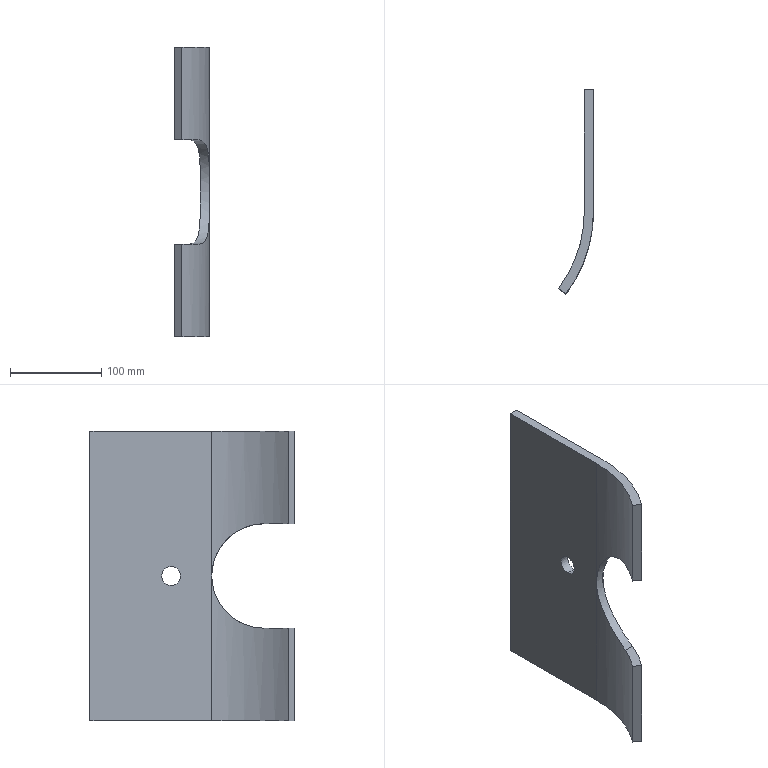Part | SolidWorks | features Extrusion 1, ICE 1 | 1 solid | 16 faces | box 38.131 x 223.442 x 317.5 mm | volume 624053 mm3 | plane 9 | cylinder 7 | commonest cylinder face diameters 20.574 x2 279.4 x2 299.4 x2 114.3 x1
STEP:
#1=CARTESIAN_POINT('',(-10.,0.,10.287));
#2=VERTEX_POINT('',#1);
#3=CARTESIAN_POINT('',(-10.,0.,-10.287));
#4=VERTEX_POINT('',#3);
#5=CARTESIAN_POINT('',(-10.,0.,0.));
#6=DIRECTION('',(1.,0.,0.));
#7=DIRECTION('',(0.,1.,0.));
#8=AXIS2_PLACEMENT_3D('',#5,#6,#7);
#9=CIRCLE('',#8,10.287);
#10=EDGE_CURVE('',#2,#4,#9,.T.);
#11=ORIENTED_EDGE('',*,*,#10,.F.);
#12=CARTESIAN_POINT('',(0.,0.,10.287));
#13=VERTEX_POINT('',#12);
#14=CARTESIAN_POINT('',(-184.15,0.,10.287));
#15=DIRECTION('',(1.,0.,0.));
#16=VECTOR('',#15,1000.);
#17=LINE('',#14,#16);
#18=EDGE_CURVE('',#2,#13,#17,.T.);
#19=ORIENTED_EDGE('',*,*,#18,.T.);
#20=CARTESIAN_POINT('',(0.,0.,-10.287));
#21=VERTEX_POINT('',#20);
#22=CARTESIAN_POINT('',(0.,0.,0.));
#23=DIRECTION('',(-1.,0.,0.));
#24=DIRECTION('',(0.,-1.,0.));
#25=AXIS2_PLACEMENT_3D('',#22,#23,#24);
#26=CIRCLE('',#25,10.287);
#27=EDGE_CURVE('',#21,#13,#26,.T.);
#28=ORIENTED_EDGE('',*,*,#27,.F.);
#29=CARTESIAN_POINT('',(-184.15,0.,-10.287));
#30=DIRECTION('',(1.,0.,0.));
#31=VECTOR('',#30,1000.);
#32=LINE('',#29,#31);
#33=EDGE_CURVE('',#4,#21,#32,.T.);
#34=ORIENTED_EDGE('',*,*,#33,.F.);
#35=EDGE_LOOP('',(#11,#19,#28,#34));
#36=FACE_OUTER_BOUND('',#35,.T.);
#37=CARTESIAN_POINT('',(-184.15,0.,0.));
#38=DIRECTION('',(1.,0.,0.));
#39=DIRECTION('',(0.,0.,-1.));
#40=AXIS2_PLACEMENT_3D('',#37,#38,#39);
#41=CYLINDRICAL_SURFACE('',#40,10.287);
#42=ADVANCED_FACE('',(#36),#41,.F.);
#43=CARTESIAN_POINT('',(-38.131,-128.524,-57.15));
#44=VERTEX_POINT('',#43);
#45=CARTESIAN_POINT('',(-38.131,-128.524,-158.75));
#46=VERTEX_POINT('',#45);
#47=CARTESIAN_POINT('',(-38.131,-128.524,158.75));
#48=DIRECTION('',(0.,0.,-1.));
#49=VECTOR('',#48,1000.);
#50=LINE('',#47,#49);
#51=EDGE_CURVE('',#44,#46,#50,.T.);
#52=ORIENTED_EDGE('',*,*,#51,.F.);
#53=CARTESIAN_POINT('',(-22.225,-101.6,-57.15));
#54=VERTEX_POINT('',#53);
#55=CARTESIAN_POINT('',(-149.7,-44.45,-57.15));
#56=DIRECTION('',(0.,0.,1.));
#57=DIRECTION('',(0.,1.,0.));
#58=AXIS2_PLACEMENT_3D('',#55,#56,#57);
#59=CIRCLE('',#58,139.7);
#60=EDGE_CURVE('',#44,#54,#59,.T.);
#61=ORIENTED_EDGE('',*,*,#60,.T.);
#62=CARTESIAN_POINT('',(-10.,-44.45,0.));
#63=VERTEX_POINT('',#62);
#64=CARTESIAN_POINT('',(-22.225,-101.6,-57.15));
#65=CARTESIAN_POINT('',(-20.653,-98.094,-57.15));
#66=CARTESIAN_POINT('',(-19.249,-94.576,-56.83));
#67=CARTESIAN_POINT('',(-17.38,-89.293,-55.838));
#68=CARTESIAN_POINT('',(-16.796,-87.531,-55.422));
#69=CARTESIAN_POINT('',(-15.978,-84.889,-54.66));
#70=CARTESIAN_POINT('',(-15.714,-84.006,-54.382));
#71=CARTESIAN_POINT('',(-15.209,-82.255,-53.784));
#72=CARTESIAN_POINT('',(-14.969,-81.387,-53.464));
#73=CARTESIAN_POINT('',(-13.82,-77.092,-51.76));
#74=CARTESIAN_POINT('',(-13.077,-73.786,-50.067));
#75=CARTESIAN_POINT('',(-12.324,-69.838,-47.52));
#76=CARTESIAN_POINT('',(-12.182,-69.057,-46.989));
#77=CARTESIAN_POINT('',(-11.915,-67.516,-45.883));
#78=CARTESIAN_POINT('',(-11.79,-66.753,-45.307));
#79=CARTESIAN_POINT('',(-11.441,-64.523,-43.532));
#80=CARTESIAN_POINT('',(-11.244,-63.102,-42.28));
#81=CARTESIAN_POINT('',(-10.906,-60.393,-39.644));
#82=CARTESIAN_POINT('',(-10.765,-59.104,-38.259));
#83=CARTESIAN_POINT('',(-10.588,-57.27,-36.082));
#84=CARTESIAN_POINT('',(-10.535,-56.676,-35.339));
#85=CARTESIAN_POINT('',(-10.438,-55.522,-33.82));
#86=CARTESIAN_POINT('',(-10.395,-54.96,-33.042));
#87=CARTESIAN_POINT('',(-10.201,-52.253,-29.081));
#88=CARTESIAN_POINT('',(-10.12,-50.436,-25.745));
#89=CARTESIAN_POINT('',(-10.049,-48.219,-20.499));
#90=CARTESIAN_POINT('',(-10.034,-47.565,-18.709));
#91=CARTESIAN_POINT('',(-10.018,-46.716,-15.963));
#92=CARTESIAN_POINT('',(-10.014,-46.455,-15.036));
#93=CARTESIAN_POINT('',(-10.008,-45.983,-13.181));
#94=CARTESIAN_POINT('',(-10.006,-45.77,-12.251));
#95=CARTESIAN_POINT('',(-9.998,-44.828,-7.588));
#96=CARTESIAN_POINT('',(-10.,-44.45,-3.815));
#97=CARTESIAN_POINT('',(-10.,-44.45,0.));
#98=B_SPLINE_CURVE_WITH_KNOTS('',3,(#64,#65,#66,#67,#68,#69,#70,#71,#72,#73,#74,#75,#76,#77,#78,#79,#80,#81,#82,#83,#84,#85,#86,#87,#88,#89,#90,#91,#92,#93,#94,#95,#96,#97),.UNSPECIFIED.,.F.,.F.,(4,2,2,2,2,2,2,2,2,2,2,2,2,2,2,2,4),(0.,0.01138,0.01706,0.01991,0.02275,0.03413,0.03697,0.03982,0.0455,0.05119,0.05404,0.05688,0.06826,0.07394,0.07679,0.07963,0.09101),.UNSPECIFIED.);
#99=EDGE_CURVE('',#54,#63,#98,.T.);
#100=ORIENTED_EDGE('',*,*,#99,.T.);
#101=CARTESIAN_POINT('',(-10.,-44.45,-158.75));
#102=VERTEX_POINT('',#101);
#103=CARTESIAN_POINT('',(-10.,-44.45,158.75));
#104=DIRECTION('',(0.,0.,-1.));
#105=VECTOR('',#104,1000.);
#106=LINE('',#103,#105);
#107=EDGE_CURVE('',#63,#102,#106,.T.);
#108=ORIENTED_EDGE('',*,*,#107,.T.);
#109=CARTESIAN_POINT('',(-149.7,-44.45,-158.75));
#110=DIRECTION('',(0.,0.,-1.));
#111=DIRECTION('',(1.,0.,0.));
#112=AXIS2_PLACEMENT_3D('',#109,#110,#111);
#113=CIRCLE('',#112,139.7);
#114=EDGE_CURVE('',#102,#46,#113,.T.);
#115=ORIENTED_EDGE('',*,*,#114,.T.);
#116=EDGE_LOOP('',(#52,#61,#100,#108,#115));
#117=FACE_OUTER_BOUND('',#116,.T.);
#118=CARTESIAN_POINT('',(-149.7,-44.45,158.75));
#119=DIRECTION('',(0.,0.,-1.));
#120=DIRECTION('',(-1.,0.,0.));
#121=AXIS2_PLACEMENT_3D('',#118,#119,#120);
#122=CYLINDRICAL_SURFACE('',#121,139.7);
#123=ADVANCED_FACE('',(#117),#122,.F.);
#124=CARTESIAN_POINT('',(-30.144,-134.542,-57.15));
#125=VERTEX_POINT('',#124);
#126=CARTESIAN_POINT('',(-30.144,-134.542,-158.75));
#127=VERTEX_POINT('',#126);
#128=CARTESIAN_POINT('',(-30.144,-134.542,158.75));
#129=DIRECTION('',(0.,0.,-1.));
#130=VECTOR('',#129,1000.);
#131=LINE('',#128,#130);
#132=EDGE_CURVE('',#125,#127,#131,.T.);
#133=ORIENTED_EDGE('',*,*,#132,.F.);
#134=CARTESIAN_POINT('',(-30.144,-134.542,-57.15));
#135=DIRECTION('',(-0.7986,0.6018,0.));
#136=VECTOR('',#135,1000.);
#137=LINE('',#134,#136);
#138=EDGE_CURVE('',#125,#44,#137,.T.);
#139=ORIENTED_EDGE('',*,*,#138,.T.);
#140=ORIENTED_EDGE('',*,*,#51,.T.);
#141=CARTESIAN_POINT('',(-30.144,-134.542,-158.75));
#142=DIRECTION('',(0.7986,-0.6018,0.));
#143=VECTOR('',#142,1000.);
#144=LINE('',#141,#143);
#145=EDGE_CURVE('',#46,#127,#144,.T.);
#146=ORIENTED_EDGE('',*,*,#145,.T.);
#147=EDGE_LOOP('',(#133,#139,#140,#146));
#148=FACE_OUTER_BOUND('',#147,.T.);
#149=CARTESIAN_POINT('',(-30.144,-134.542,158.75));
#150=DIRECTION('',(0.6018,0.7986,0.));
#151=DIRECTION('',(-0.7986,0.6018,0.));
#152=AXIS2_PLACEMENT_3D('',#149,#150,#151);
#153=PLANE('',#152);
#154=ADVANCED_FACE('',(#148),#153,.F.);
#155=CARTESIAN_POINT('',(0.,-44.45,0.));
#156=VERTEX_POINT('',#155);
#157=CARTESIAN_POINT('',(-11.338,-101.6,-57.15));
#158=VERTEX_POINT('',#157);
#159=CARTESIAN_POINT('',(0.,-44.45,0.));
#160=CARTESIAN_POINT('',(0.,-44.45,-0.9496));
#161=CARTESIAN_POINT('',(0.000005753,-44.474,-1.902));
#162=CARTESIAN_POINT('',(-0.00003983,-44.569,-3.811));
#163=CARTESIAN_POINT('',(-0.00009177,-44.641,-4.767));
#164=CARTESIAN_POINT('',(-0.0006387,-44.927,-7.611));
#165=CARTESIAN_POINT('',(-0.001464,-45.211,-9.485));
#166=CARTESIAN_POINT('',(-0.009996,-46.335,-15.041));
#167=CARTESIAN_POINT('',(-0.0226,-47.446,-18.66));
#168=CARTESIAN_POINT('',(-0.08943,-49.677,-23.954));
#169=CARTESIAN_POINT('',(-0.1197,-50.504,-25.669));
#170=CARTESIAN_POINT('',(-0.204,-52.314,-28.994));
#171=CARTESIAN_POINT('',(-0.2579,-53.298,-30.605));
#172=CARTESIAN_POINT('',(-0.3989,-55.423,-33.725));
#173=CARTESIAN_POINT('',(-0.4859,-56.564,-35.235));
#174=CARTESIAN_POINT('',(-0.6497,-58.395,-37.421));
#175=CARTESIAN_POINT('',(-0.7099,-59.027,-38.139));
#176=CARTESIAN_POINT('',(-0.8426,-60.324,-39.539));
#177=CARTESIAN_POINT('',(-0.9146,-60.987,-40.219));
#178=CARTESIAN_POINT('',(-1.307,-64.373,-43.527));
#179=CARTESIAN_POINT('',(-1.72,-67.305,-45.87));
#180=CARTESIAN_POINT('',(-2.414,-71.237,-48.426));
#181=CARTESIAN_POINT('',(-2.562,-72.037,-48.919));
#182=CARTESIAN_POINT('',(-2.876,-73.664,-49.866));
#183=CARTESIAN_POINT('',(-3.043,-74.493,-50.321));
#184=CARTESIAN_POINT('',(-3.57,-76.993,-51.615));
#185=CARTESIAN_POINT('',(-3.956,-78.683,-52.386));
#186=CARTESIAN_POINT('',(-5.226,-83.817,-54.438));
#187=CARTESIAN_POINT('',(-6.222,-87.325,-55.459));
#188=CARTESIAN_POINT('',(-7.976,-92.7,-56.482));
#189=CARTESIAN_POINT('',(-8.598,-94.489,-56.734));
#190=CARTESIAN_POINT('',(-9.913,-98.053,-57.068));
#191=CARTESIAN_POINT('',(-10.607,-99.83,-57.15));
#192=CARTESIAN_POINT('',(-11.338,-101.6,-57.15));
#193=B_SPLINE_CURVE_WITH_KNOTS('',3,(#159,#160,#161,#162,#163,#164,#165,#166,#167,#168,#169,#170,#171,#172,#173,#174,#175,#176,#177,#178,#179,#180,#181,#182,#183,#184,#185,#186,#187,#188,#189,#190,#191,#192),.UNSPECIFIED.,.F.,.F.,(4,2,2,2,2,2,2,2,2,2,2,2,2,2,2,2,4),(0.09078,0.09361,0.09645,0.1021,0.1135,0.1191,0.1248,0.1305,0.1333,0.1361,0.1475,0.1503,0.1531,0.1588,0.1701,0.1758,0.1815),.UNSPECIFIED.);
#194=EDGE_CURVE('',#156,#158,#193,.T.);
#195=ORIENTED_EDGE('',*,*,#194,.T.);
#196=CARTESIAN_POINT('',(-149.7,-44.45,-57.15));
#197=DIRECTION('',(0.,0.,-1.));
#198=DIRECTION('',(0.,1.,0.));
#199=AXIS2_PLACEMENT_3D('',#196,#197,#198);
#200=CIRCLE('',#199,149.7);
#201=EDGE_CURVE('',#158,#125,#200,.T.);
#202=ORIENTED_EDGE('',*,*,#201,.T.);
#203=ORIENTED_EDGE('',*,*,#132,.T.);
#204=CARTESIAN_POINT('',(0.,-44.45,-158.75));
#205=VERTEX_POINT('',#204);
#206=CARTESIAN_POINT('',(-149.7,-44.45,-158.75));
#207=DIRECTION('',(0.,0.,1.));
#208=DIRECTION('',(1.,0.,0.));
#209=AXIS2_PLACEMENT_3D('',#206,#207,#208);
#210=CIRCLE('',#209,149.7);
#211=EDGE_CURVE('',#127,#205,#210,.T.);
#212=ORIENTED_EDGE('',*,*,#211,.T.);
#213=CARTESIAN_POINT('',(0.,-44.45,158.75));
#214=DIRECTION('',(0.,0.,-1.));
#215=VECTOR('',#214,1000.);
#216=LINE('',#213,#215);
#217=EDGE_CURVE('',#156,#205,#216,.T.);
#218=ORIENTED_EDGE('',*,*,#217,.F.);
#219=EDGE_LOOP('',(#195,#202,#203,#212,#218));
#220=FACE_OUTER_BOUND('',#219,.T.);
#221=CARTESIAN_POINT('',(-149.7,-44.45,158.75));
#222=DIRECTION('',(0.,0.,-1.));
#223=DIRECTION('',(-1.,0.,0.));
#224=AXIS2_PLACEMENT_3D('',#221,#222,#223);
#225=CYLINDRICAL_SURFACE('',#224,149.7);
#226=ADVANCED_FACE('',(#220),#225,.T.);
#227=CARTESIAN_POINT('',(-10.,0.,0.));
#228=DIRECTION('',(1.,0.,0.));
#229=DIRECTION('',(0.,1.,0.));
#230=AXIS2_PLACEMENT_3D('',#227,#228,#229);
#231=CIRCLE('',#230,10.287);
#232=EDGE_CURVE('',#4,#2,#231,.T.);
#233=ORIENTED_EDGE('',*,*,#232,.T.);
#234=ORIENTED_EDGE('',*,*,#10,.T.);
#235=EDGE_LOOP('',(#233,#234));
#236=FACE_BOUND('',#235,.T.);
#237=CARTESIAN_POINT('',(-10.,88.9,-158.75));
#238=VERTEX_POINT('',#237);
#239=CARTESIAN_POINT('',(-10.,88.9,-158.75));
#240=DIRECTION('',(0.,-1.,0.));
#241=VECTOR('',#240,1000.);
#242=LINE('',#239,#241);
#243=EDGE_CURVE('',#238,#102,#242,.T.);
#244=ORIENTED_EDGE('',*,*,#243,.T.);
#245=ORIENTED_EDGE('',*,*,#107,.F.);
#246=CARTESIAN_POINT('',(-10.,-44.45,158.75));
#247=VERTEX_POINT('',#246);
#248=CARTESIAN_POINT('',(-10.,-44.45,158.75));
#249=DIRECTION('',(0.,0.,-1.));
#250=VECTOR('',#249,1000.);
#251=LINE('',#248,#250);
#252=EDGE_CURVE('',#247,#63,#251,.T.);
#253=ORIENTED_EDGE('',*,*,#252,.F.);
#254=CARTESIAN_POINT('',(-10.,88.9,158.75));
#255=VERTEX_POINT('',#254);
#256=CARTESIAN_POINT('',(-10.,88.9,158.75));
#257=DIRECTION('',(0.,-1.,0.));
#258=VECTOR('',#257,1000.);
#259=LINE('',#256,#258);
#260=EDGE_CURVE('',#255,#247,#259,.T.);
#261=ORIENTED_EDGE('',*,*,#260,.F.);
#262=CARTESIAN_POINT('',(-10.,88.9,158.75));
#263=DIRECTION('',(0.,0.,-1.));
#264=VECTOR('',#263,1000.);
#265=LINE('',#262,#264);
#266=EDGE_CURVE('',#255,#238,#265,.T.);
#267=ORIENTED_EDGE('',*,*,#266,.T.);
#268=EDGE_LOOP('',(#244,#245,#253,#261,#267));
#269=FACE_OUTER_BOUND('',#268,.T.);
#270=CARTESIAN_POINT('',(-10.,88.9,158.75));
#271=DIRECTION('',(1.,0.,0.));
#272=DIRECTION('',(0.,1.,0.));
#273=AXIS2_PLACEMENT_3D('',#270,#271,#272);
#274=PLANE('',#273);
#275=ADVANCED_FACE('',(#236,#269),#274,.F.);
#276=ORIENTED_EDGE('',*,*,#252,.T.);
#277=CARTESIAN_POINT('',(-22.225,-101.6,57.15));
#278=VERTEX_POINT('',#277);
#279=CARTESIAN_POINT('',(-10.,-44.45,0.));
#280=CARTESIAN_POINT('',(-10.,-44.45,0.9528));
#281=CARTESIAN_POINT('',(-10.,-44.474,1.908));
#282=CARTESIAN_POINT('',(-10.,-44.57,3.825));
#283=CARTESIAN_POINT('',(-10.,-44.642,4.781));
#284=CARTESIAN_POINT('',(-10.001,-44.929,7.629));
#285=CARTESIAN_POINT('',(-10.002,-45.214,9.506));
#286=CARTESIAN_POINT('',(-10.008,-45.967,13.218));
#287=CARTESIAN_POINT('',(-10.013,-46.436,15.054));
#288=CARTESIAN_POINT('',(-10.028,-47.276,17.775));
#289=CARTESIAN_POINT('',(-10.035,-47.579,18.677));
#290=CARTESIAN_POINT('',(-10.051,-48.233,20.47));
#291=CARTESIAN_POINT('',(-10.061,-48.584,21.362));
#292=CARTESIAN_POINT('',(-10.121,-50.451,25.78));
#293=CARTESIAN_POINT('',(-10.203,-52.272,29.107));
#294=CARTESIAN_POINT('',(-10.432,-55.475,33.796));
#295=CARTESIAN_POINT('',(-10.526,-56.621,35.308));
#296=CARTESIAN_POINT('',(-10.703,-58.463,37.499));
#297=CARTESIAN_POINT('',(-10.769,-59.099,38.219));
#298=CARTESIAN_POINT('',(-10.912,-60.399,39.617));
#299=CARTESIAN_POINT('',(-10.99,-61.064,40.297));
#300=CARTESIAN_POINT('',(-11.413,-64.459,43.601));
#301=CARTESIAN_POINT('',(-11.861,-67.4,45.941));
#302=CARTESIAN_POINT('',(-12.611,-71.345,48.493));
#303=CARTESIAN_POINT('',(-12.771,-72.147,48.985));
#304=CARTESIAN_POINT('',(-13.111,-73.779,49.93));
#305=CARTESIAN_POINT('',(-13.292,-74.609,50.383));
#306=CARTESIAN_POINT('',(-13.86,-77.107,51.669));
#307=CARTESIAN_POINT('',(-14.276,-78.795,52.435));
#308=CARTESIAN_POINT('',(-15.189,-82.214,53.793));
#309=CARTESIAN_POINT('',(-15.686,-83.944,54.385));
#310=CARTESIAN_POINT('',(-16.497,-86.568,55.145));
#311=CARTESIAN_POINT('',(-16.778,-87.448,55.377));
#312=CARTESIAN_POINT('',(-17.363,-89.216,55.799));
#313=CARTESIAN_POINT('',(-17.668,-90.106,55.99));
#314=CARTESIAN_POINT('',(-19.241,-94.559,56.83));
#315=CARTESIAN_POINT('',(-20.653,-98.095,57.15));
#316=CARTESIAN_POINT('',(-22.225,-101.6,57.15));
#317=B_SPLINE_CURVE_WITH_KNOTS('',3,(#279,#280,#281,#282,#283,#284,#285,#286,#287,#288,#289,#290,#291,#292,#293,#294,#295,#296,#297,#298,#299,#300,#301,#302,#303,#304,#305,#306,#307,#308,#309,#310,#311,#312,#313,#314,#315,#316),.UNSPECIFIED.,.F.,.F.,(4,2,2,2,2,2,2,2,2,2,2,2,2,2,2,2,2,2,4),(0.09101,0.09385,0.09669,0.1024,0.1081,0.1109,0.1137,0.1251,0.1308,0.1336,0.1365,0.1478,0.1507,0.1535,0.1592,0.1649,0.1677,0.1706,0.1819),.UNSPECIFIED.);
#318=EDGE_CURVE('',#63,#278,#317,.T.);
#319=ORIENTED_EDGE('',*,*,#318,.T.);
#320=CARTESIAN_POINT('',(-38.131,-128.524,57.15));
#321=VERTEX_POINT('',#320);
#322=CARTESIAN_POINT('',(-149.7,-44.45,57.15));
#323=DIRECTION('',(0.,0.,-1.));
#324=DIRECTION('',(0.,-1.,0.));
#325=AXIS2_PLACEMENT_3D('',#322,#323,#324);
#326=CIRCLE('',#325,139.7);
#327=EDGE_CURVE('',#278,#321,#326,.T.);
#328=ORIENTED_EDGE('',*,*,#327,.T.);
#329=CARTESIAN_POINT('',(-38.131,-128.524,158.75));
#330=VERTEX_POINT('',#329);
#331=CARTESIAN_POINT('',(-38.131,-128.524,158.75));
#332=DIRECTION('',(0.,0.,-1.));
#333=VECTOR('',#332,1000.);
#334=LINE('',#331,#333);
#335=EDGE_CURVE('',#330,#321,#334,.T.);
#336=ORIENTED_EDGE('',*,*,#335,.F.);
#337=CARTESIAN_POINT('',(-149.7,-44.45,158.75));
#338=DIRECTION('',(0.,0.,-1.));
#339=DIRECTION('',(1.,0.,0.));
#340=AXIS2_PLACEMENT_3D('',#337,#338,#339);
#341=CIRCLE('',#340,139.7);
#342=EDGE_CURVE('',#247,#330,#341,.T.);
#343=ORIENTED_EDGE('',*,*,#342,.F.);
#344=EDGE_LOOP('',(#276,#319,#328,#336,#343));
#345=FACE_OUTER_BOUND('',#344,.T.);
#346=CARTESIAN_POINT('',(-149.7,-44.45,158.75));
#347=DIRECTION('',(0.,0.,-1.));
#348=DIRECTION('',(-1.,0.,0.));
#349=AXIS2_PLACEMENT_3D('',#346,#347,#348);
#350=CYLINDRICAL_SURFACE('',#349,139.7);
#351=ADVANCED_FACE('',(#345),#350,.F.);
#352=ORIENTED_EDGE('',*,*,#335,.T.);
#353=CARTESIAN_POINT('',(-30.144,-134.542,57.15));
#354=VERTEX_POINT('',#353);
#355=CARTESIAN_POINT('',(-30.144,-134.542,57.15));
#356=DIRECTION('',(0.7986,-0.6018,0.));
#357=VECTOR('',#356,1000.);
#358=LINE('',#355,#357);
#359=EDGE_CURVE('',#321,#354,#358,.T.);
#360=ORIENTED_EDGE('',*,*,#359,.T.);
#361=CARTESIAN_POINT('',(-30.144,-134.542,158.75));
#362=VERTEX_POINT('',#361);
#363=CARTESIAN_POINT('',(-30.144,-134.542,158.75));
#364=DIRECTION('',(0.,0.,-1.));
#365=VECTOR('',#364,1000.);
#366=LINE('',#363,#365);
#367=EDGE_CURVE('',#362,#354,#366,.T.);
#368=ORIENTED_EDGE('',*,*,#367,.F.);
#369=CARTESIAN_POINT('',(-30.144,-134.542,158.75));
#370=DIRECTION('',(0.7986,-0.6018,0.));
#371=VECTOR('',#370,1000.);
#372=LINE('',#369,#371);
#373=EDGE_CURVE('',#330,#362,#372,.T.);
#374=ORIENTED_EDGE('',*,*,#373,.F.);
#375=EDGE_LOOP('',(#352,#360,#368,#374));
#376=FACE_OUTER_BOUND('',#375,.T.);
#377=CARTESIAN_POINT('',(-30.144,-134.542,158.75));
#378=DIRECTION('',(0.6018,0.7986,0.));
#379=DIRECTION('',(-0.7986,0.6018,0.));
#380=AXIS2_PLACEMENT_3D('',#377,#378,#379);
#381=PLANE('',#380);
#382=ADVANCED_FACE('',(#376),#381,.F.);
#383=CARTESIAN_POINT('',(-11.338,-101.6,57.15));
#384=VERTEX_POINT('',#383);
#385=CARTESIAN_POINT('',(-149.7,-44.45,57.15));
#386=DIRECTION('',(0.,0.,1.));
#387=DIRECTION('',(0.,-1.,0.));
#388=AXIS2_PLACEMENT_3D('',#385,#386,#387);
#389=CIRCLE('',#388,149.7);
#390=EDGE_CURVE('',#354,#384,#389,.T.);
#391=ORIENTED_EDGE('',*,*,#390,.T.);
#392=CARTESIAN_POINT('',(-11.338,-101.6,57.15));
#393=CARTESIAN_POINT('',(-9.875,-98.057,57.15));
#394=CARTESIAN_POINT('',(-8.57,-94.512,56.823));
#395=CARTESIAN_POINT('',(-6.834,-89.202,55.818));
#396=CARTESIAN_POINT('',(-6.292,-87.433,55.397));
#397=CARTESIAN_POINT('',(-5.533,-84.784,54.628));
#398=CARTESIAN_POINT('',(-5.288,-83.899,54.347));
#399=CARTESIAN_POINT('',(-4.82,-82.144,53.744));
#400=CARTESIAN_POINT('',(-4.597,-81.275,53.422));
#401=CARTESIAN_POINT('',(-3.533,-76.974,51.705));
#402=CARTESIAN_POINT('',(-2.845,-73.672,50.003));
#403=CARTESIAN_POINT('',(-2.148,-69.733,47.45));
#404=CARTESIAN_POINT('',(-2.017,-68.954,46.918));
#405=CARTESIAN_POINT('',(-1.77,-67.417,45.81));
#406=CARTESIAN_POINT('',(-1.654,-66.657,45.233));
#407=CARTESIAN_POINT('',(-1.332,-64.433,43.455));
#408=CARTESIAN_POINT('',(-1.15,-63.017,42.202));
#409=CARTESIAN_POINT('',(-0.6808,-58.968,38.247));
#410=CARTESIAN_POINT('',(-0.4725,-56.53,35.348));
#411=CARTESIAN_POINT('',(-0.1858,-52.214,29.014));
#412=CARTESIAN_POINT('',(-0.1113,-50.405,25.682));
#413=CARTESIAN_POINT('',(-0.04517,-48.2,20.449));
#414=CARTESIAN_POINT('',(-0.03104,-47.55,18.664));
#415=CARTESIAN_POINT('',(-0.01673,-46.706,15.927));
#416=CARTESIAN_POINT('',(-0.01312,-46.446,15.002));
#417=CARTESIAN_POINT('',(-0.007584,-45.975,13.149));
#418=CARTESIAN_POINT('',(-0.005648,-45.764,12.221));
#419=CARTESIAN_POINT('',(0.00141,-44.826,7.566));
#420=CARTESIAN_POINT('',(0.,-44.45,3.802));
#421=CARTESIAN_POINT('',(0.,-44.45,0.));
#422=B_SPLINE_CURVE_WITH_KNOTS('',3,(#392,#393,#394,#395,#396,#397,#398,#399,#400,#401,#402,#403,#404,#405,#406,#407,#408,#409,#410,#411,#412,#413,#414,#415,#416,#417,#418,#419,#420,#421),.UNSPECIFIED.,.F.,.F.,(4,2,2,2,2,2,2,2,2,2,2,2,2,2,4),(0.,0.01135,0.01702,0.01986,0.0227,0.03404,0.03688,0.03972,0.04539,0.05674,0.06809,0.07376,0.0766,0.07943,0.09078),.UNSPECIFIED.);
#423=EDGE_CURVE('',#384,#156,#422,.T.);
#424=ORIENTED_EDGE('',*,*,#423,.T.);
#425=CARTESIAN_POINT('',(0.,-44.45,158.75));
#426=VERTEX_POINT('',#425);
#427=CARTESIAN_POINT('',(0.,-44.45,158.75));
#428=DIRECTION('',(0.,0.,-1.));
#429=VECTOR('',#428,1000.);
#430=LINE('',#427,#429);
#431=EDGE_CURVE('',#426,#156,#430,.T.);
#432=ORIENTED_EDGE('',*,*,#431,.F.);
#433=CARTESIAN_POINT('',(-149.7,-44.45,158.75));
#434=DIRECTION('',(0.,0.,1.));
#435=DIRECTION('',(1.,0.,0.));
#436=AXIS2_PLACEMENT_3D('',#433,#434,#435);
#437=CIRCLE('',#436,149.7);
#438=EDGE_CURVE('',#362,#426,#437,.T.);
#439=ORIENTED_EDGE('',*,*,#438,.F.);
#440=ORIENTED_EDGE('',*,*,#367,.T.);
#441=EDGE_LOOP('',(#391,#424,#432,#439,#440));
#442=FACE_OUTER_BOUND('',#441,.T.);
#443=CARTESIAN_POINT('',(-149.7,-44.45,158.75));
#444=DIRECTION('',(0.,0.,-1.));
#445=DIRECTION('',(-1.,0.,0.));
#446=AXIS2_PLACEMENT_3D('',#443,#444,#445);
#447=CYLINDRICAL_SURFACE('',#446,149.7);
#448=ADVANCED_FACE('',(#442),#447,.T.);
#449=ORIENTED_EDGE('',*,*,#27,.T.);
#450=CARTESIAN_POINT('',(0.,0.,0.));
#451=DIRECTION('',(-1.,0.,0.));
#452=DIRECTION('',(0.,-1.,0.));
#453=AXIS2_PLACEMENT_3D('',#450,#451,#452);
#454=CIRCLE('',#453,10.287);
#455=EDGE_CURVE('',#13,#21,#454,.T.);
#456=ORIENTED_EDGE('',*,*,#455,.T.);
#457=EDGE_LOOP('',(#449,#456));
#458=FACE_BOUND('',#457,.T.);
#459=CARTESIAN_POINT('',(0.,88.9,-158.75));
#460=VERTEX_POINT('',#459);
#461=CARTESIAN_POINT('',(0.,88.9,-158.75));
#462=DIRECTION('',(0.,1.,0.));
#463=VECTOR('',#462,1000.);
#464=LINE('',#461,#463);
#465=EDGE_CURVE('',#205,#460,#464,.T.);
#466=ORIENTED_EDGE('',*,*,#465,.T.);
#467=CARTESIAN_POINT('',(0.,88.9,158.75));
#468=VERTEX_POINT('',#467);
#469=CARTESIAN_POINT('',(0.,88.9,158.75));
#470=DIRECTION('',(0.,0.,-1.));
#471=VECTOR('',#470,1000.);
#472=LINE('',#469,#471);
#473=EDGE_CURVE('',#468,#460,#472,.T.);
#474=ORIENTED_EDGE('',*,*,#473,.F.);
#475=CARTESIAN_POINT('',(0.,88.9,158.75));
#476=DIRECTION('',(0.,1.,0.));
#477=VECTOR('',#476,1000.);
#478=LINE('',#475,#477);
#479=EDGE_CURVE('',#426,#468,#478,.T.);
#480=ORIENTED_EDGE('',*,*,#479,.F.);
#481=ORIENTED_EDGE('',*,*,#431,.T.);
#482=ORIENTED_EDGE('',*,*,#217,.T.);
#483=EDGE_LOOP('',(#466,#474,#480,#481,#482));
#484=FACE_OUTER_BOUND('',#483,.T.);
#485=CARTESIAN_POINT('',(0.,88.9,158.75));
#486=DIRECTION('',(-1.,0.,0.));
#487=DIRECTION('',(0.,-1.,0.));
#488=AXIS2_PLACEMENT_3D('',#485,#486,#487);
#489=PLANE('',#488);
#490=ADVANCED_FACE('',(#458,#484),#489,.F.);
#491=CARTESIAN_POINT('',(-10.,88.9,-158.75));
#492=DIRECTION('',(-1.,0.,0.));
#493=VECTOR('',#492,1000.);
#494=LINE('',#491,#493);
#495=EDGE_CURVE('',#460,#238,#494,.T.);
#496=ORIENTED_EDGE('',*,*,#495,.T.);
#497=ORIENTED_EDGE('',*,*,#266,.F.);
#498=CARTESIAN_POINT('',(-10.,88.9,158.75));
#499=DIRECTION('',(-1.,0.,0.));
#500=VECTOR('',#499,1000.);
#501=LINE('',#498,#500);
#502=EDGE_CURVE('',#468,#255,#501,.T.);
#503=ORIENTED_EDGE('',*,*,#502,.F.);
#504=ORIENTED_EDGE('',*,*,#473,.T.);
#505=EDGE_LOOP('',(#496,#497,#503,#504));
#506=FACE_OUTER_BOUND('',#505,.T.);
#507=CARTESIAN_POINT('',(-10.,88.9,158.75));
#508=DIRECTION('',(0.,-1.,0.));
#509=DIRECTION('',(0.,0.,-1.));
#510=AXIS2_PLACEMENT_3D('',#507,#508,#509);
#511=PLANE('',#510);
#512=ADVANCED_FACE('',(#506),#511,.F.);
#513=ORIENTED_EDGE('',*,*,#260,.T.);
#514=ORIENTED_EDGE('',*,*,#342,.T.);
#515=ORIENTED_EDGE('',*,*,#373,.T.);
#516=ORIENTED_EDGE('',*,*,#438,.T.);
#517=ORIENTED_EDGE('',*,*,#479,.T.);
#518=ORIENTED_EDGE('',*,*,#502,.T.);
#519=EDGE_LOOP('',(#513,#514,#515,#516,#517,#518));
#520=FACE_OUTER_BOUND('',#519,.T.);
#521=CARTESIAN_POINT('',(-149.7,-44.45,158.75));
#522=DIRECTION('',(0.,0.,1.));
#523=DIRECTION('',(1.,0.,0.));
#524=AXIS2_PLACEMENT_3D('',#521,#522,#523);
#525=PLANE('',#524);
#526=ADVANCED_FACE('',(#520),#525,.T.);
#527=ORIENTED_EDGE('',*,*,#243,.F.);
#528=ORIENTED_EDGE('',*,*,#495,.F.);
#529=ORIENTED_EDGE('',*,*,#465,.F.);
#530=ORIENTED_EDGE('',*,*,#211,.F.);
#531=ORIENTED_EDGE('',*,*,#145,.F.);
#532=ORIENTED_EDGE('',*,*,#114,.F.);
#533=EDGE_LOOP('',(#527,#528,#529,#530,#531,#532));
#534=FACE_OUTER_BOUND('',#533,.T.);
#535=CARTESIAN_POINT('',(-149.7,-44.45,-158.75));
#536=DIRECTION('',(0.,0.,1.));
#537=DIRECTION('',(1.,0.,0.));
#538=AXIS2_PLACEMENT_3D('',#535,#536,#537);
#539=PLANE('',#538);
#540=ADVANCED_FACE('',(#534),#539,.F.);
#541=ORIENTED_EDGE('',*,*,#18,.F.);
#542=ORIENTED_EDGE('',*,*,#232,.F.);
#543=ORIENTED_EDGE('',*,*,#33,.T.);
#544=ORIENTED_EDGE('',*,*,#455,.F.);
#545=EDGE_LOOP('',(#541,#542,#543,#544));
#546=FACE_OUTER_BOUND('',#545,.T.);
#547=CARTESIAN_POINT('',(-184.15,0.,0.));
#548=DIRECTION('',(1.,0.,0.));
#549=DIRECTION('',(0.,0.,-1.));
#550=AXIS2_PLACEMENT_3D('',#547,#548,#549);
#551=CYLINDRICAL_SURFACE('',#550,10.287);
#552=ADVANCED_FACE('',(#546),#551,.F.);
#553=ORIENTED_EDGE('',*,*,#138,.F.);
#554=ORIENTED_EDGE('',*,*,#201,.F.);
#555=CARTESIAN_POINT('',(-184.15,-101.6,-57.15));
#556=DIRECTION('',(1.,0.,0.));
#557=VECTOR('',#556,1000.);
#558=LINE('',#555,#557);
#559=EDGE_CURVE('',#54,#158,#558,.T.);
#560=ORIENTED_EDGE('',*,*,#559,.F.);
#561=ORIENTED_EDGE('',*,*,#60,.F.);
#562=EDGE_LOOP('',(#553,#554,#560,#561));
#563=FACE_OUTER_BOUND('',#562,.T.);
#564=CARTESIAN_POINT('',(-184.15,-134.542,-57.15));
#565=DIRECTION('',(0.,0.,-1.));
#566=DIRECTION('',(0.,1.,0.));
#567=AXIS2_PLACEMENT_3D('',#564,#565,#566);
#568=PLANE('',#567);
#569=ADVANCED_FACE('',(#563),#568,.F.);
#570=CARTESIAN_POINT('',(-184.15,-101.6,57.15));
#571=DIRECTION('',(1.,0.,0.));
#572=VECTOR('',#571,1000.);
#573=LINE('',#570,#572);
#574=EDGE_CURVE('',#278,#384,#573,.T.);
#575=ORIENTED_EDGE('',*,*,#574,.T.);
#576=ORIENTED_EDGE('',*,*,#390,.F.);
#577=ORIENTED_EDGE('',*,*,#359,.F.);
#578=ORIENTED_EDGE('',*,*,#327,.F.);
#579=EDGE_LOOP('',(#575,#576,#577,#578));
#580=FACE_OUTER_BOUND('',#579,.T.);
#581=CARTESIAN_POINT('',(-184.15,-101.6,57.15));
#582=DIRECTION('',(0.,0.,1.));
#583=DIRECTION('',(0.,-1.,0.));
#584=AXIS2_PLACEMENT_3D('',#581,#582,#583);
#585=PLANE('',#584);
#586=ADVANCED_FACE('',(#580),#585,.F.);
#587=ORIENTED_EDGE('',*,*,#559,.T.);
#588=ORIENTED_EDGE('',*,*,#194,.F.);
#589=ORIENTED_EDGE('',*,*,#423,.F.);
#590=ORIENTED_EDGE('',*,*,#574,.F.);
#591=ORIENTED_EDGE('',*,*,#318,.F.);
#592=ORIENTED_EDGE('',*,*,#99,.F.);
#593=EDGE_LOOP('',(#587,#588,#589,#590,#591,#592));
#594=FACE_OUTER_BOUND('',#593,.T.);
#595=CARTESIAN_POINT('',(-184.15,-101.6,0.));
#596=DIRECTION('',(1.,0.,0.));
#597=DIRECTION('',(0.,0.,-1.));
#598=AXIS2_PLACEMENT_3D('',#595,#596,#597);
#599=CYLINDRICAL_SURFACE('',#598,57.15);
#600=ADVANCED_FACE('',(#594),#599,.F.);
#601=CLOSED_SHELL('',(#42,#123,#154,#226,#275,#351,#382,#448,#490,#512,#526,#540,#552,#569,#586,#600));
#602=MANIFOLD_SOLID_BREP('',#601);
#603=CARTESIAN_POINT('',(0.,0.,0.));
#604=DIRECTION('',(0.,0.,1.));
#605=DIRECTION('',(1.,0.,0.));
#606=AXIS2_PLACEMENT_3D('',#603,#604,#605);
#607=(LENGTH_UNIT()NAMED_UNIT(*)SI_UNIT(.MILLI.,.METRE.));
#608=UNCERTAINTY_MEASURE_WITH_UNIT(LENGTH_MEASURE(0.00001),#607,'','');
#609=(NAMED_UNIT(*)PLANE_ANGLE_UNIT()SI_UNIT($,.RADIAN.));
#610=(NAMED_UNIT(*)SI_UNIT($,.STERADIAN.)SOLID_ANGLE_UNIT());
#611=(GEOMETRIC_REPRESENTATION_CONTEXT(3)GLOBAL_UNCERTAINTY_ASSIGNED_CONTEXT((#608))GLOBAL_UNIT_ASSIGNED_CONTEXT((#607,#609,#610))REPRESENTATION_CONTEXT('',''));
#612=ADVANCED_BREP_SHAPE_REPRESENTATION('',(#602,#606),#611);